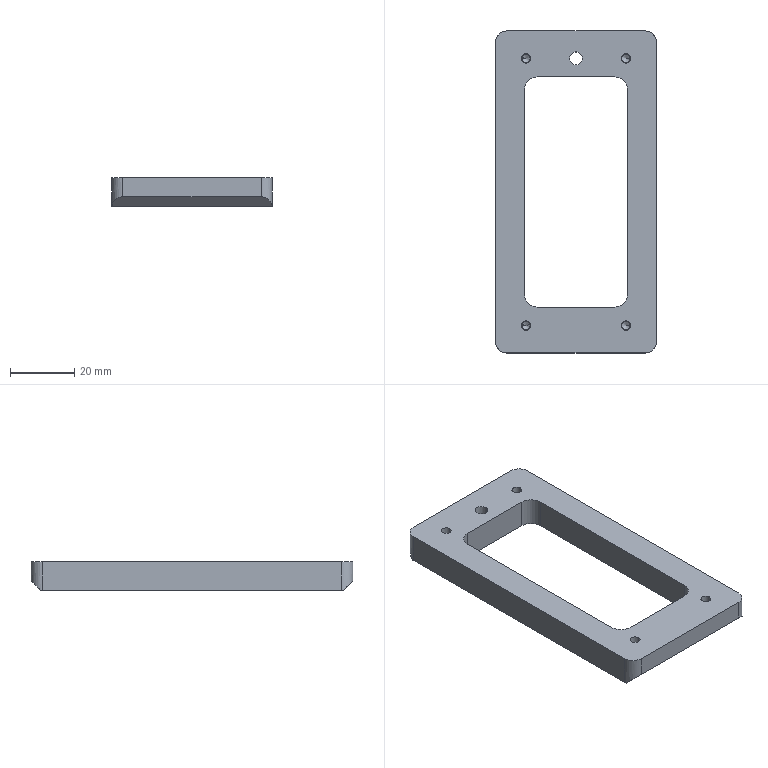Part | STEP file | X77-02213 [2] | 1 solid | 50 faces | box 50 x 100 x 9 mm | volume 23719 mm3 | cylinder 26 | plane 16 | cone 8 | commonest cylinder face diameters 2.5 x8 3 x8 7.116 x4 8 x4 4 x2
STEP:
#1=CARTESIAN_POINT('',(2.,41.5,0.));
#2=VERTEX_POINT('',#1);
#3=CARTESIAN_POINT('',(-2.,41.5,0.));
#4=VERTEX_POINT('',#3);
#5=CARTESIAN_POINT('',(-0.000000005,41.5,0.));
#6=DIRECTION('',(0.,0.,1.));
#7=DIRECTION('',(-1.,0.,0.));
#8=AXIS2_PLACEMENT_3D('',#5,#6,#7);
#9=CIRCLE('',#8,2.);
#10=EDGE_CURVE('',#2,#4,#9,.T.);
#11=ORIENTED_EDGE('',*,*,#10,.F.);
#12=CARTESIAN_POINT('',(2.,41.5,9.));
#13=VERTEX_POINT('',#12);
#14=CARTESIAN_POINT('',(2.,41.5,0.));
#15=DIRECTION('',(0.,0.,1.));
#16=VECTOR('',#15,1000.);
#17=LINE('',#14,#16);
#18=EDGE_CURVE('',#2,#13,#17,.T.);
#19=ORIENTED_EDGE('',*,*,#18,.T.);
#20=CARTESIAN_POINT('',(-2.,41.5,9.));
#21=VERTEX_POINT('',#20);
#22=CARTESIAN_POINT('',(-0.000000005,41.5,9.));
#23=DIRECTION('',(0.,0.,-1.));
#24=DIRECTION('',(-1.,0.,0.));
#25=AXIS2_PLACEMENT_3D('',#22,#23,#24);
#26=CIRCLE('',#25,2.);
#27=EDGE_CURVE('',#21,#13,#26,.T.);
#28=ORIENTED_EDGE('',*,*,#27,.F.);
#29=CARTESIAN_POINT('',(-2.,41.5,0.));
#30=DIRECTION('',(0.,0.,1.));
#31=VECTOR('',#30,1000.);
#32=LINE('',#29,#31);
#33=EDGE_CURVE('',#4,#21,#32,.T.);
#34=ORIENTED_EDGE('',*,*,#33,.F.);
#35=EDGE_LOOP('',(#11,#19,#28,#34));
#36=FACE_OUTER_BOUND('',#35,.T.);
#37=CARTESIAN_POINT('',(-0.000000005,41.5,0.));
#38=DIRECTION('',(0.,0.,1.));
#39=DIRECTION('',(-1.,0.,0.));
#40=AXIS2_PLACEMENT_3D('',#37,#38,#39);
#41=CYLINDRICAL_SURFACE('',#40,2.);
#42=ADVANCED_FACE('',(#36),#41,.F.);
#43=CARTESIAN_POINT('',(-14.001,-41.5,4.));
#44=VERTEX_POINT('',#43);
#45=CARTESIAN_POINT('',(-17.001,-41.5,4.));
#46=VERTEX_POINT('',#45);
#47=CARTESIAN_POINT('',(-15.501,-41.5,4.));
#48=DIRECTION('',(0.,0.,1.));
#49=DIRECTION('',(-1.,0.,0.));
#50=AXIS2_PLACEMENT_3D('',#47,#48,#49);
#51=CIRCLE('',#50,1.5);
#52=EDGE_CURVE('',#44,#46,#51,.T.);
#53=ORIENTED_EDGE('',*,*,#52,.F.);
#54=CARTESIAN_POINT('',(-14.001,-41.5,9.));
#55=VERTEX_POINT('',#54);
#56=CARTESIAN_POINT('',(-14.001,-41.5,10.));
#57=DIRECTION('',(0.,0.,1.));
#58=VECTOR('',#57,1000.);
#59=LINE('',#56,#58);
#60=EDGE_CURVE('',#44,#55,#59,.T.);
#61=ORIENTED_EDGE('',*,*,#60,.T.);
#62=CARTESIAN_POINT('',(-17.001,-41.5,9.));
#63=VERTEX_POINT('',#62);
#64=CARTESIAN_POINT('',(-15.501,-41.5,9.));
#65=DIRECTION('',(0.,0.,-1.));
#66=DIRECTION('',(-1.,0.,0.));
#67=AXIS2_PLACEMENT_3D('',#64,#65,#66);
#68=CIRCLE('',#67,1.5);
#69=EDGE_CURVE('',#63,#55,#68,.T.);
#70=ORIENTED_EDGE('',*,*,#69,.F.);
#71=CARTESIAN_POINT('',(-17.001,-41.5,10.));
#72=DIRECTION('',(0.,0.,1.));
#73=VECTOR('',#72,1000.);
#74=LINE('',#71,#73);
#75=EDGE_CURVE('',#46,#63,#74,.T.);
#76=ORIENTED_EDGE('',*,*,#75,.F.);
#77=EDGE_LOOP('',(#53,#61,#70,#76));
#78=FACE_OUTER_BOUND('',#77,.T.);
#79=CARTESIAN_POINT('',(-15.501,-41.5,10.));
#80=DIRECTION('',(0.,0.,1.));
#81=DIRECTION('',(-1.,0.,0.));
#82=AXIS2_PLACEMENT_3D('',#79,#80,#81);
#83=CYLINDRICAL_SURFACE('',#82,1.5);
#84=ADVANCED_FACE('',(#78),#83,.F.);
#85=CARTESIAN_POINT('',(-14.251,-41.5,2.5));
#86=VERTEX_POINT('',#85);
#87=CARTESIAN_POINT('',(-16.751,-41.5,2.5));
#88=VERTEX_POINT('',#87);
#89=CARTESIAN_POINT('',(-15.501,-41.5,2.5));
#90=DIRECTION('',(0.,0.,1.));
#91=DIRECTION('',(-1.,0.,0.));
#92=AXIS2_PLACEMENT_3D('',#89,#90,#91);
#93=CIRCLE('',#92,1.25);
#94=EDGE_CURVE('',#86,#88,#93,.T.);
#95=ORIENTED_EDGE('',*,*,#94,.F.);
#96=CARTESIAN_POINT('',(-14.251,-41.5,4.));
#97=VERTEX_POINT('',#96);
#98=CARTESIAN_POINT('',(-14.251,-41.5,10.));
#99=DIRECTION('',(0.,0.,1.));
#100=VECTOR('',#99,1000.);
#101=LINE('',#98,#100);
#102=EDGE_CURVE('',#86,#97,#101,.T.);
#103=ORIENTED_EDGE('',*,*,#102,.T.);
#104=CARTESIAN_POINT('',(-16.751,-41.5,4.));
#105=VERTEX_POINT('',#104);
#106=CARTESIAN_POINT('',(-15.501,-41.5,4.));
#107=DIRECTION('',(0.,0.,1.));
#108=DIRECTION('',(-1.,0.,0.));
#109=AXIS2_PLACEMENT_3D('',#106,#107,#108);
#110=CIRCLE('',#109,1.25);
#111=EDGE_CURVE('',#97,#105,#110,.T.);
#112=ORIENTED_EDGE('',*,*,#111,.T.);
#113=CARTESIAN_POINT('',(-16.751,-41.5,10.));
#114=DIRECTION('',(0.,0.,1.));
#115=VECTOR('',#114,1000.);
#116=LINE('',#113,#115);
#117=EDGE_CURVE('',#88,#105,#116,.T.);
#118=ORIENTED_EDGE('',*,*,#117,.F.);
#119=EDGE_LOOP('',(#95,#103,#112,#118));
#120=FACE_OUTER_BOUND('',#119,.T.);
#121=CARTESIAN_POINT('',(-15.501,-41.5,10.));
#122=DIRECTION('',(0.,0.,1.));
#123=DIRECTION('',(-1.,0.,0.));
#124=AXIS2_PLACEMENT_3D('',#121,#122,#123);
#125=CYLINDRICAL_SURFACE('',#124,1.25);
#126=ADVANCED_FACE('',(#120),#125,.F.);
#127=CARTESIAN_POINT('',(-15.501,-41.5,1.749));
#128=VERTEX_POINT('',#127);
#129=CARTESIAN_POINT('',(-16.751,-41.5,2.5));
#130=DIRECTION('',(-0.8572,0.,0.515));
#131=VECTOR('',#130,1000.);
#132=LINE('',#129,#131);
#133=EDGE_CURVE('',#128,#88,#132,.T.);
#134=ORIENTED_EDGE('',*,*,#133,.F.);
#135=CARTESIAN_POINT('',(-14.251,-41.5,2.5));
#136=DIRECTION('',(0.8572,0.,0.515));
#137=VECTOR('',#136,1000.);
#138=LINE('',#135,#137);
#139=EDGE_CURVE('',#128,#86,#138,.T.);
#140=ORIENTED_EDGE('',*,*,#139,.T.);
#141=ORIENTED_EDGE('',*,*,#94,.T.);
#142=EDGE_LOOP('',(#134,#140,#141));
#143=FACE_OUTER_BOUND('',#142,.T.);
#144=CARTESIAN_POINT('',(-15.501,-41.5,2.5));
#145=DIRECTION('',(0.,0.,1.));
#146=DIRECTION('',(-1.,0.,0.));
#147=AXIS2_PLACEMENT_3D('',#144,#145,#146);
#148=CONICAL_SURFACE('',#147,1.25,1.03);
#149=ADVANCED_FACE('',(#143),#148,.F.);
#150=CARTESIAN_POINT('',(-14.005,41.5,4.));
#151=VERTEX_POINT('',#150);
#152=CARTESIAN_POINT('',(-17.005,41.5,4.));
#153=VERTEX_POINT('',#152);
#154=CARTESIAN_POINT('',(-15.505,41.5,4.));
#155=DIRECTION('',(0.,0.,1.));
#156=DIRECTION('',(-1.,0.,0.));
#157=AXIS2_PLACEMENT_3D('',#154,#155,#156);
#158=CIRCLE('',#157,1.5);
#159=EDGE_CURVE('',#151,#153,#158,.T.);
#160=ORIENTED_EDGE('',*,*,#159,.F.);
#161=CARTESIAN_POINT('',(-14.005,41.5,9.));
#162=VERTEX_POINT('',#161);
#163=CARTESIAN_POINT('',(-14.005,41.5,10.));
#164=DIRECTION('',(0.,0.,1.));
#165=VECTOR('',#164,1000.);
#166=LINE('',#163,#165);
#167=EDGE_CURVE('',#151,#162,#166,.T.);
#168=ORIENTED_EDGE('',*,*,#167,.T.);
#169=CARTESIAN_POINT('',(-17.005,41.5,9.));
#170=VERTEX_POINT('',#169);
#171=CARTESIAN_POINT('',(-15.505,41.5,9.));
#172=DIRECTION('',(0.,0.,-1.));
#173=DIRECTION('',(-1.,0.,0.));
#174=AXIS2_PLACEMENT_3D('',#171,#172,#173);
#175=CIRCLE('',#174,1.5);
#176=EDGE_CURVE('',#170,#162,#175,.T.);
#177=ORIENTED_EDGE('',*,*,#176,.F.);
#178=CARTESIAN_POINT('',(-17.005,41.5,10.));
#179=DIRECTION('',(0.,0.,1.));
#180=VECTOR('',#179,1000.);
#181=LINE('',#178,#180);
#182=EDGE_CURVE('',#153,#170,#181,.T.);
#183=ORIENTED_EDGE('',*,*,#182,.F.);
#184=EDGE_LOOP('',(#160,#168,#177,#183));
#185=FACE_OUTER_BOUND('',#184,.T.);
#186=CARTESIAN_POINT('',(-15.505,41.5,10.));
#187=DIRECTION('',(0.,0.,1.));
#188=DIRECTION('',(-1.,0.,0.));
#189=AXIS2_PLACEMENT_3D('',#186,#187,#188);
#190=CYLINDRICAL_SURFACE('',#189,1.5);
#191=ADVANCED_FACE('',(#185),#190,.F.);
#192=CARTESIAN_POINT('',(-14.255,41.5,2.5));
#193=VERTEX_POINT('',#192);
#194=CARTESIAN_POINT('',(-16.755,41.5,2.5));
#195=VERTEX_POINT('',#194);
#196=CARTESIAN_POINT('',(-15.505,41.5,2.5));
#197=DIRECTION('',(0.,0.,1.));
#198=DIRECTION('',(-1.,0.,0.));
#199=AXIS2_PLACEMENT_3D('',#196,#197,#198);
#200=CIRCLE('',#199,1.25);
#201=EDGE_CURVE('',#193,#195,#200,.T.);
#202=ORIENTED_EDGE('',*,*,#201,.F.);
#203=CARTESIAN_POINT('',(-14.255,41.5,4.));
#204=VERTEX_POINT('',#203);
#205=CARTESIAN_POINT('',(-14.255,41.5,10.));
#206=DIRECTION('',(0.,0.,1.));
#207=VECTOR('',#206,1000.);
#208=LINE('',#205,#207);
#209=EDGE_CURVE('',#193,#204,#208,.T.);
#210=ORIENTED_EDGE('',*,*,#209,.T.);
#211=CARTESIAN_POINT('',(-16.755,41.5,4.));
#212=VERTEX_POINT('',#211);
#213=CARTESIAN_POINT('',(-15.505,41.5,4.));
#214=DIRECTION('',(0.,0.,1.));
#215=DIRECTION('',(-1.,0.,0.));
#216=AXIS2_PLACEMENT_3D('',#213,#214,#215);
#217=CIRCLE('',#216,1.25);
#218=EDGE_CURVE('',#204,#212,#217,.T.);
#219=ORIENTED_EDGE('',*,*,#218,.T.);
#220=CARTESIAN_POINT('',(-16.755,41.5,10.));
#221=DIRECTION('',(0.,0.,1.));
#222=VECTOR('',#221,1000.);
#223=LINE('',#220,#222);
#224=EDGE_CURVE('',#195,#212,#223,.T.);
#225=ORIENTED_EDGE('',*,*,#224,.F.);
#226=EDGE_LOOP('',(#202,#210,#219,#225));
#227=FACE_OUTER_BOUND('',#226,.T.);
#228=CARTESIAN_POINT('',(-15.505,41.5,10.));
#229=DIRECTION('',(0.,0.,1.));
#230=DIRECTION('',(-1.,0.,0.));
#231=AXIS2_PLACEMENT_3D('',#228,#229,#230);
#232=CYLINDRICAL_SURFACE('',#231,1.25);
#233=ADVANCED_FACE('',(#227),#232,.F.);
#234=CARTESIAN_POINT('',(-15.505,41.5,1.749));
#235=VERTEX_POINT('',#234);
#236=CARTESIAN_POINT('',(-16.755,41.5,2.5));
#237=DIRECTION('',(-0.8572,0.,0.515));
#238=VECTOR('',#237,1000.);
#239=LINE('',#236,#238);
#240=EDGE_CURVE('',#235,#195,#239,.T.);
#241=ORIENTED_EDGE('',*,*,#240,.F.);
#242=CARTESIAN_POINT('',(-14.255,41.5,2.5));
#243=DIRECTION('',(0.8572,0.,0.515));
#244=VECTOR('',#243,1000.);
#245=LINE('',#242,#244);
#246=EDGE_CURVE('',#235,#193,#245,.T.);
#247=ORIENTED_EDGE('',*,*,#246,.T.);
#248=ORIENTED_EDGE('',*,*,#201,.T.);
#249=EDGE_LOOP('',(#241,#247,#248));
#250=FACE_OUTER_BOUND('',#249,.T.);
#251=CARTESIAN_POINT('',(-15.505,41.5,2.5));
#252=DIRECTION('',(0.,0.,1.));
#253=DIRECTION('',(-1.,0.,0.));
#254=AXIS2_PLACEMENT_3D('',#251,#252,#253);
#255=CONICAL_SURFACE('',#254,1.25,1.03);
#256=ADVANCED_FACE('',(#250),#255,.F.);
#257=CARTESIAN_POINT('',(16.999,41.5,4.));
#258=VERTEX_POINT('',#257);
#259=CARTESIAN_POINT('',(13.999,41.5,4.));
#260=VERTEX_POINT('',#259);
#261=CARTESIAN_POINT('',(15.499,41.5,4.));
#262=DIRECTION('',(0.,0.,1.));
#263=DIRECTION('',(-1.,0.,0.));
#264=AXIS2_PLACEMENT_3D('',#261,#262,#263);
#265=CIRCLE('',#264,1.5);
#266=EDGE_CURVE('',#258,#260,#265,.T.);
#267=ORIENTED_EDGE('',*,*,#266,.F.);
#268=CARTESIAN_POINT('',(16.999,41.5,9.));
#269=VERTEX_POINT('',#268);
#270=CARTESIAN_POINT('',(16.999,41.5,10.));
#271=DIRECTION('',(0.,0.,1.));
#272=VECTOR('',#271,1000.);
#273=LINE('',#270,#272);
#274=EDGE_CURVE('',#258,#269,#273,.T.);
#275=ORIENTED_EDGE('',*,*,#274,.T.);
#276=CARTESIAN_POINT('',(13.999,41.5,9.));
#277=VERTEX_POINT('',#276);
#278=CARTESIAN_POINT('',(15.499,41.5,9.));
#279=DIRECTION('',(0.,0.,-1.));
#280=DIRECTION('',(-1.,0.,0.));
#281=AXIS2_PLACEMENT_3D('',#278,#279,#280);
#282=CIRCLE('',#281,1.5);
#283=EDGE_CURVE('',#277,#269,#282,.T.);
#284=ORIENTED_EDGE('',*,*,#283,.F.);
#285=CARTESIAN_POINT('',(13.999,41.5,10.));
#286=DIRECTION('',(0.,0.,1.));
#287=VECTOR('',#286,1000.);
#288=LINE('',#285,#287);
#289=EDGE_CURVE('',#260,#277,#288,.T.);
#290=ORIENTED_EDGE('',*,*,#289,.F.);
#291=EDGE_LOOP('',(#267,#275,#284,#290));
#292=FACE_OUTER_BOUND('',#291,.T.);
#293=CARTESIAN_POINT('',(15.499,41.5,10.));
#294=DIRECTION('',(0.,0.,1.));
#295=DIRECTION('',(-1.,0.,0.));
#296=AXIS2_PLACEMENT_3D('',#293,#294,#295);
#297=CYLINDRICAL_SURFACE('',#296,1.5);
#298=ADVANCED_FACE('',(#292),#297,.F.);
#299=CARTESIAN_POINT('',(16.749,41.5,2.5));
#300=VERTEX_POINT('',#299);
#301=CARTESIAN_POINT('',(14.249,41.5,2.5));
#302=VERTEX_POINT('',#301);
#303=CARTESIAN_POINT('',(15.499,41.5,2.5));
#304=DIRECTION('',(0.,0.,1.));
#305=DIRECTION('',(-1.,0.,0.));
#306=AXIS2_PLACEMENT_3D('',#303,#304,#305);
#307=CIRCLE('',#306,1.25);
#308=EDGE_CURVE('',#300,#302,#307,.T.);
#309=ORIENTED_EDGE('',*,*,#308,.F.);
#310=CARTESIAN_POINT('',(16.749,41.5,4.));
#311=VERTEX_POINT('',#310);
#312=CARTESIAN_POINT('',(16.749,41.5,10.));
#313=DIRECTION('',(0.,0.,1.));
#314=VECTOR('',#313,1000.);
#315=LINE('',#312,#314);
#316=EDGE_CURVE('',#300,#311,#315,.T.);
#317=ORIENTED_EDGE('',*,*,#316,.T.);
#318=CARTESIAN_POINT('',(14.249,41.5,4.));
#319=VERTEX_POINT('',#318);
#320=CARTESIAN_POINT('',(15.499,41.5,4.));
#321=DIRECTION('',(0.,0.,1.));
#322=DIRECTION('',(-1.,0.,0.));
#323=AXIS2_PLACEMENT_3D('',#320,#321,#322);
#324=CIRCLE('',#323,1.25);
#325=EDGE_CURVE('',#311,#319,#324,.T.);
#326=ORIENTED_EDGE('',*,*,#325,.T.);
#327=CARTESIAN_POINT('',(14.249,41.5,10.));
#328=DIRECTION('',(0.,0.,1.));
#329=VECTOR('',#328,1000.);
#330=LINE('',#327,#329);
#331=EDGE_CURVE('',#302,#319,#330,.T.);
#332=ORIENTED_EDGE('',*,*,#331,.F.);
#333=EDGE_LOOP('',(#309,#317,#326,#332));
#334=FACE_OUTER_BOUND('',#333,.T.);
#335=CARTESIAN_POINT('',(15.499,41.5,10.));
#336=DIRECTION('',(0.,0.,1.));
#337=DIRECTION('',(-1.,0.,0.));
#338=AXIS2_PLACEMENT_3D('',#335,#336,#337);
#339=CYLINDRICAL_SURFACE('',#338,1.25);
#340=ADVANCED_FACE('',(#334),#339,.F.);
#341=CARTESIAN_POINT('',(15.499,41.5,1.749));
#342=VERTEX_POINT('',#341);
#343=CARTESIAN_POINT('',(14.249,41.5,2.5));
#344=DIRECTION('',(-0.8572,0.,0.515));
#345=VECTOR('',#344,1000.);
#346=LINE('',#343,#345);
#347=EDGE_CURVE('',#342,#302,#346,.T.);
#348=ORIENTED_EDGE('',*,*,#347,.F.);
#349=CARTESIAN_POINT('',(16.749,41.5,2.5));
#350=DIRECTION('',(0.8572,0.,0.515));
#351=VECTOR('',#350,1000.);
#352=LINE('',#349,#351);
#353=EDGE_CURVE('',#342,#300,#352,.T.);
#354=ORIENTED_EDGE('',*,*,#353,.T.);
#355=ORIENTED_EDGE('',*,*,#308,.T.);
#356=EDGE_LOOP('',(#348,#354,#355));
#357=FACE_OUTER_BOUND('',#356,.T.);
#358=CARTESIAN_POINT('',(15.499,41.5,2.5));
#359=DIRECTION('',(0.,0.,1.));
#360=DIRECTION('',(-1.,0.,0.));
#361=AXIS2_PLACEMENT_3D('',#358,#359,#360);
#362=CONICAL_SURFACE('',#361,1.25,1.03);
#363=ADVANCED_FACE('',(#357),#362,.F.);
#364=CARTESIAN_POINT('',(16.75,-41.5,2.5));
#365=VERTEX_POINT('',#364);
#366=CARTESIAN_POINT('',(14.25,-41.5,2.5));
#367=VERTEX_POINT('',#366);
#368=CARTESIAN_POINT('',(15.5,-41.5,2.5));
#369=DIRECTION('',(0.,0.,1.));
#370=DIRECTION('',(-1.,0.,0.));
#371=AXIS2_PLACEMENT_3D('',#368,#369,#370);
#372=CIRCLE('',#371,1.25);
#373=EDGE_CURVE('',#365,#367,#372,.T.);
#374=ORIENTED_EDGE('',*,*,#373,.F.);
#375=CARTESIAN_POINT('',(16.75,-41.5,4.));
#376=VERTEX_POINT('',#375);
#377=CARTESIAN_POINT('',(16.75,-41.5,10.));
#378=DIRECTION('',(0.,0.,1.));
#379=VECTOR('',#378,1000.);
#380=LINE('',#377,#379);
#381=EDGE_CURVE('',#365,#376,#380,.T.);
#382=ORIENTED_EDGE('',*,*,#381,.T.);
#383=CARTESIAN_POINT('',(14.25,-41.5,4.));
#384=VERTEX_POINT('',#383);
#385=CARTESIAN_POINT('',(15.5,-41.5,4.));
#386=DIRECTION('',(0.,0.,1.));
#387=DIRECTION('',(-1.,0.,0.));
#388=AXIS2_PLACEMENT_3D('',#385,#386,#387);
#389=CIRCLE('',#388,1.25);
#390=EDGE_CURVE('',#376,#384,#389,.T.);
#391=ORIENTED_EDGE('',*,*,#390,.T.);
#392=CARTESIAN_POINT('',(14.25,-41.5,10.));
#393=DIRECTION('',(0.,0.,1.));
#394=VECTOR('',#393,1000.);
#395=LINE('',#392,#394);
#396=EDGE_CURVE('',#367,#384,#395,.T.);
#397=ORIENTED_EDGE('',*,*,#396,.F.);
#398=EDGE_LOOP('',(#374,#382,#391,#397));
#399=FACE_OUTER_BOUND('',#398,.T.);
#400=CARTESIAN_POINT('',(15.5,-41.5,10.));
#401=DIRECTION('',(0.,0.,1.));
#402=DIRECTION('',(-1.,0.,0.));
#403=AXIS2_PLACEMENT_3D('',#400,#401,#402);
#404=CYLINDRICAL_SURFACE('',#403,1.25);
#405=ADVANCED_FACE('',(#399),#404,.F.);
#406=CARTESIAN_POINT('',(15.5,-41.5,1.749));
#407=VERTEX_POINT('',#406);
#408=CARTESIAN_POINT('',(14.25,-41.5,2.5));
#409=DIRECTION('',(-0.8572,0.,0.515));
#410=VECTOR('',#409,1000.);
#411=LINE('',#408,#410);
#412=EDGE_CURVE('',#407,#367,#411,.T.);
#413=ORIENTED_EDGE('',*,*,#412,.F.);
#414=CARTESIAN_POINT('',(16.75,-41.5,2.5));
#415=DIRECTION('',(0.8572,0.,0.515));
#416=VECTOR('',#415,1000.);
#417=LINE('',#414,#416);
#418=EDGE_CURVE('',#407,#365,#417,.T.);
#419=ORIENTED_EDGE('',*,*,#418,.T.);
#420=ORIENTED_EDGE('',*,*,#373,.T.);
#421=EDGE_LOOP('',(#413,#419,#420));
#422=FACE_OUTER_BOUND('',#421,.T.);
#423=CARTESIAN_POINT('',(15.5,-41.5,2.5));
#424=DIRECTION('',(0.,0.,1.));
#425=DIRECTION('',(-1.,0.,0.));
#426=AXIS2_PLACEMENT_3D('',#423,#424,#425);
#427=CONICAL_SURFACE('',#426,1.25,1.03);
#428=ADVANCED_FACE('',(#422),#427,.F.);
#429=CARTESIAN_POINT('',(17.,-41.5,4.));
#430=VERTEX_POINT('',#429);
#431=CARTESIAN_POINT('',(14.,-41.5,4.));
#432=VERTEX_POINT('',#431);
#433=CARTESIAN_POINT('',(15.5,-41.5,4.));
#434=DIRECTION('',(0.,0.,1.));
#435=DIRECTION('',(-1.,0.,0.));
#436=AXIS2_PLACEMENT_3D('',#433,#434,#435);
#437=CIRCLE('',#436,1.5);
#438=EDGE_CURVE('',#430,#432,#437,.T.);
#439=ORIENTED_EDGE('',*,*,#438,.F.);
#440=CARTESIAN_POINT('',(17.,-41.5,9.));
#441=VERTEX_POINT('',#440);
#442=CARTESIAN_POINT('',(17.,-41.5,10.));
#443=DIRECTION('',(0.,0.,1.));
#444=VECTOR('',#443,1000.);
#445=LINE('',#442,#444);
#446=EDGE_CURVE('',#430,#441,#445,.T.);
#447=ORIENTED_EDGE('',*,*,#446,.T.);
#448=CARTESIAN_POINT('',(14.,-41.5,9.));
#449=VERTEX_POINT('',#448);
#450=CARTESIAN_POINT('',(15.5,-41.5,9.));
#451=DIRECTION('',(0.,0.,-1.));
#452=DIRECTION('',(-1.,0.,0.));
#453=AXIS2_PLACEMENT_3D('',#450,#451,#452);
#454=CIRCLE('',#453,1.5);
#455=EDGE_CURVE('',#449,#441,#454,.T.);
#456=ORIENTED_EDGE('',*,*,#455,.F.);
#457=CARTESIAN_POINT('',(14.,-41.5,10.));
#458=DIRECTION('',(0.,0.,1.));
#459=VECTOR('',#458,1000.);
#460=LINE('',#457,#459);
#461=EDGE_CURVE('',#432,#449,#460,.T.);
#462=ORIENTED_EDGE('',*,*,#461,.F.);
#463=EDGE_LOOP('',(#439,#447,#456,#462));
#464=FACE_OUTER_BOUND('',#463,.T.);
#465=CARTESIAN_POINT('',(15.5,-41.5,10.));
#466=DIRECTION('',(0.,0.,1.));
#467=DIRECTION('',(-1.,0.,0.));
#468=AXIS2_PLACEMENT_3D('',#465,#466,#467);
#469=CYLINDRICAL_SURFACE('',#468,1.5);
#470=ADVANCED_FACE('',(#464),#469,.F.);
#471=ORIENTED_EDGE('',*,*,#446,.F.);
#472=CARTESIAN_POINT('',(15.5,-41.5,4.));
#473=DIRECTION('',(0.,0.,1.));
#474=DIRECTION('',(-1.,0.,0.));
#475=AXIS2_PLACEMENT_3D('',#472,#473,#474);
#476=CIRCLE('',#475,1.5);
#477=EDGE_CURVE('',#432,#430,#476,.T.);
#478=ORIENTED_EDGE('',*,*,#477,.F.);
#479=ORIENTED_EDGE('',*,*,#461,.T.);
#480=CARTESIAN_POINT('',(15.5,-41.5,9.));
#481=DIRECTION('',(0.,0.,-1.));
#482=DIRECTION('',(-1.,0.,0.));
#483=AXIS2_PLACEMENT_3D('',#480,#481,#482);
#484=CIRCLE('',#483,1.5);
#485=EDGE_CURVE('',#441,#449,#484,.T.);
#486=ORIENTED_EDGE('',*,*,#485,.F.);
#487=EDGE_LOOP('',(#471,#478,#479,#486));
#488=FACE_OUTER_BOUND('',#487,.T.);
#489=CARTESIAN_POINT('',(15.5,-41.5,10.));
#490=DIRECTION('',(0.,0.,1.));
#491=DIRECTION('',(-1.,0.,0.));
#492=AXIS2_PLACEMENT_3D('',#489,#490,#491);
#493=CYLINDRICAL_SURFACE('',#492,1.5);
#494=ADVANCED_FACE('',(#488),#493,.F.);
#495=ORIENTED_EDGE('',*,*,#418,.F.);
#496=ORIENTED_EDGE('',*,*,#412,.T.);
#497=CARTESIAN_POINT('',(15.5,-41.5,2.5));
#498=DIRECTION('',(0.,0.,1.));
#499=DIRECTION('',(-1.,0.,0.));
#500=AXIS2_PLACEMENT_3D('',#497,#498,#499);
#501=CIRCLE('',#500,1.25);
#502=EDGE_CURVE('',#367,#365,#501,.T.);
#503=ORIENTED_EDGE('',*,*,#502,.T.);
#504=EDGE_LOOP('',(#495,#496,#503));
#505=FACE_OUTER_BOUND('',#504,.T.);
#506=CARTESIAN_POINT('',(15.5,-41.5,2.5));
#507=DIRECTION('',(0.,0.,1.));
#508=DIRECTION('',(-1.,0.,0.));
#509=AXIS2_PLACEMENT_3D('',#506,#507,#508);
#510=CONICAL_SURFACE('',#509,1.25,1.03);
#511=ADVANCED_FACE('',(#505),#510,.F.);
#512=ORIENTED_EDGE('',*,*,#381,.F.);
#513=ORIENTED_EDGE('',*,*,#502,.F.);
#514=ORIENTED_EDGE('',*,*,#396,.T.);
#515=CARTESIAN_POINT('',(15.5,-41.5,4.));
#516=DIRECTION('',(0.,0.,1.));
#517=DIRECTION('',(-1.,0.,0.));
#518=AXIS2_PLACEMENT_3D('',#515,#516,#517);
#519=CIRCLE('',#518,1.25);
#520=EDGE_CURVE('',#384,#376,#519,.T.);
#521=ORIENTED_EDGE('',*,*,#520,.T.);
#522=EDGE_LOOP('',(#512,#513,#514,#521));
#523=FACE_OUTER_BOUND('',#522,.T.);
#524=CARTESIAN_POINT('',(15.5,-41.5,10.));
#525=DIRECTION('',(0.,0.,1.));
#526=DIRECTION('',(-1.,0.,0.));
#527=AXIS2_PLACEMENT_3D('',#524,#525,#526);
#528=CYLINDRICAL_SURFACE('',#527,1.25);
#529=ADVANCED_FACE('',(#523),#528,.F.);
#530=ORIENTED_EDGE('',*,*,#520,.F.);
#531=ORIENTED_EDGE('',*,*,#390,.F.);
#532=EDGE_LOOP('',(#530,#531));
#533=FACE_BOUND('',#532,.T.);
#534=ORIENTED_EDGE('',*,*,#477,.T.);
#535=ORIENTED_EDGE('',*,*,#438,.T.);
#536=EDGE_LOOP('',(#534,#535));
#537=FACE_OUTER_BOUND('',#536,.T.);
#538=CARTESIAN_POINT('',(15.5,-42.75,4.));
#539=DIRECTION('',(0.,0.,-1.));
#540=DIRECTION('',(1.,0.,0.));
#541=AXIS2_PLACEMENT_3D('',#538,#539,#540);
#542=PLANE('',#541);
#543=ADVANCED_FACE('',(#533,#537),#542,.F.);
#544=ORIENTED_EDGE('',*,*,#455,.T.);
#545=ORIENTED_EDGE('',*,*,#485,.T.);
#546=EDGE_LOOP('',(#544,#545));
#547=FACE_BOUND('',#546,.T.);
#548=ORIENTED_EDGE('',*,*,#69,.T.);
#549=CARTESIAN_POINT('',(-15.501,-41.5,9.));
#550=DIRECTION('',(0.,0.,-1.));
#551=DIRECTION('',(-1.,0.,0.));
#552=AXIS2_PLACEMENT_3D('',#549,#550,#551);
#553=CIRCLE('',#552,1.5);
#554=EDGE_CURVE('',#55,#63,#553,.T.);
#555=ORIENTED_EDGE('',*,*,#554,.T.);
#556=EDGE_LOOP('',(#548,#555));
#557=FACE_BOUND('',#556,.T.);
#558=ORIENTED_EDGE('',*,*,#176,.T.);
#559=CARTESIAN_POINT('',(-15.505,41.5,9.));
#560=DIRECTION('',(0.,0.,-1.));
#561=DIRECTION('',(-1.,0.,0.));
#562=AXIS2_PLACEMENT_3D('',#559,#560,#561);
#563=CIRCLE('',#562,1.5);
#564=EDGE_CURVE('',#162,#170,#563,.T.);
#565=ORIENTED_EDGE('',*,*,#564,.T.);
#566=EDGE_LOOP('',(#558,#565));
#567=FACE_BOUND('',#566,.T.);
#568=ORIENTED_EDGE('',*,*,#283,.T.);
#569=CARTESIAN_POINT('',(15.499,41.5,9.));
#570=DIRECTION('',(0.,0.,-1.));
#571=DIRECTION('',(-1.,0.,0.));
#572=AXIS2_PLACEMENT_3D('',#569,#570,#571);
#573=CIRCLE('',#572,1.5);
#574=EDGE_CURVE('',#269,#277,#573,.T.);
#575=ORIENTED_EDGE('',*,*,#574,.T.);
#576=EDGE_LOOP('',(#568,#575));
#577=FACE_BOUND('',#576,.T.);
#578=ORIENTED_EDGE('',*,*,#27,.T.);
#579=CARTESIAN_POINT('',(-0.000000005,41.5,9.));
#580=DIRECTION('',(0.,0.,-1.));
#581=DIRECTION('',(-1.,0.,0.));
#582=AXIS2_PLACEMENT_3D('',#579,#580,#581);
#583=CIRCLE('',#582,2.);
#584=EDGE_CURVE('',#13,#21,#583,.T.);
#585=ORIENTED_EDGE('',*,*,#584,.T.);
#586=EDGE_LOOP('',(#578,#585));
#587=FACE_BOUND('',#586,.T.);
#588=CARTESIAN_POINT('',(-12.,-35.75,9.));
#589=VERTEX_POINT('',#588);
#590=CARTESIAN_POINT('',(12.,-35.75,9.));
#591=VERTEX_POINT('',#590);
#592=CARTESIAN_POINT('',(-12.,-35.75,9.));
#593=DIRECTION('',(1.,0.,0.));
#594=VECTOR('',#593,1000.);
#595=LINE('',#592,#594);
#596=EDGE_CURVE('',#589,#591,#595,.T.);
#597=ORIENTED_EDGE('',*,*,#596,.F.);
#598=CARTESIAN_POINT('',(-16.,-31.75,9.));
#599=VERTEX_POINT('',#598);
#600=CARTESIAN_POINT('',(-12.,-31.75,9.));
#601=DIRECTION('',(0.,0.,1.));
#602=DIRECTION('',(-1.,0.,0.));
#603=AXIS2_PLACEMENT_3D('',#600,#601,#602);
#604=CIRCLE('',#603,4.);
#605=EDGE_CURVE('',#599,#589,#604,.T.);
#606=ORIENTED_EDGE('',*,*,#605,.F.);
#607=CARTESIAN_POINT('',(-16.,31.75,9.));
#608=VERTEX_POINT('',#607);
#609=CARTESIAN_POINT('',(-16.,-31.75,9.));
#610=DIRECTION('',(0.,-1.,0.));
#611=VECTOR('',#610,1000.);
#612=LINE('',#609,#611);
#613=EDGE_CURVE('',#608,#599,#612,.T.);
#614=ORIENTED_EDGE('',*,*,#613,.F.);
#615=CARTESIAN_POINT('',(-12.,35.75,9.));
#616=VERTEX_POINT('',#615);
#617=CARTESIAN_POINT('',(-12.,31.75,9.));
#618=DIRECTION('',(0.,0.,1.));
#619=DIRECTION('',(-1.,0.,0.));
#620=AXIS2_PLACEMENT_3D('',#617,#618,#619);
#621=CIRCLE('',#620,4.);
#622=EDGE_CURVE('',#616,#608,#621,.T.);
#623=ORIENTED_EDGE('',*,*,#622,.F.);
#624=CARTESIAN_POINT('',(12.,35.75,9.));
#625=VERTEX_POINT('',#624);
#626=CARTESIAN_POINT('',(-12.,35.75,9.));
#627=DIRECTION('',(-1.,0.,0.));
#628=VECTOR('',#627,1000.);
#629=LINE('',#626,#628);
#630=EDGE_CURVE('',#625,#616,#629,.T.);
#631=ORIENTED_EDGE('',*,*,#630,.F.);
#632=CARTESIAN_POINT('',(16.,31.75,9.));
#633=VERTEX_POINT('',#632);
#634=CARTESIAN_POINT('',(12.,31.75,9.));
#635=DIRECTION('',(0.,0.,1.));
#636=DIRECTION('',(-1.,0.,0.));
#637=AXIS2_PLACEMENT_3D('',#634,#635,#636);
#638=CIRCLE('',#637,4.);
#639=EDGE_CURVE('',#633,#625,#638,.T.);
#640=ORIENTED_EDGE('',*,*,#639,.F.);
#641=CARTESIAN_POINT('',(16.,-31.75,9.));
#642=VERTEX_POINT('',#641);
#643=CARTESIAN_POINT('',(16.,-31.75,9.));
#644=DIRECTION('',(0.,1.,0.));
#645=VECTOR('',#644,1000.);
#646=LINE('',#643,#645);
#647=EDGE_CURVE('',#642,#633,#646,.T.);
#648=ORIENTED_EDGE('',*,*,#647,.F.);
#649=CARTESIAN_POINT('',(12.,-31.75,9.));
#650=DIRECTION('',(0.,0.,1.));
#651=DIRECTION('',(-1.,0.,0.));
#652=AXIS2_PLACEMENT_3D('',#649,#650,#651);
#653=CIRCLE('',#652,4.);
#654=EDGE_CURVE('',#591,#642,#653,.T.);
#655=ORIENTED_EDGE('',*,*,#654,.F.);
#656=EDGE_LOOP('',(#597,#606,#614,#623,#631,#640,#648,#655));
#657=FACE_BOUND('',#656,.T.);
#658=CARTESIAN_POINT('',(25.,46.442,9.));
#659=VERTEX_POINT('',#658);
#660=CARTESIAN_POINT('',(21.442,50.,9.));
#661=VERTEX_POINT('',#660);
#662=CARTESIAN_POINT('',(21.442,46.442,9.));
#663=DIRECTION('',(0.,0.,1.));
#664=DIRECTION('',(-1.,0.,0.));
#665=AXIS2_PLACEMENT_3D('',#662,#663,#664);
#666=CIRCLE('',#665,3.558);
#667=EDGE_CURVE('',#659,#661,#666,.T.);
#668=ORIENTED_EDGE('',*,*,#667,.T.);
#669=CARTESIAN_POINT('',(-21.442,50.,9.));
#670=VERTEX_POINT('',#669);
#671=CARTESIAN_POINT('',(-21.442,50.,9.));
#672=DIRECTION('',(-1.,0.,0.));
#673=VECTOR('',#672,1000.);
#674=LINE('',#671,#673);
#675=EDGE_CURVE('',#661,#670,#674,.T.);
#676=ORIENTED_EDGE('',*,*,#675,.T.);
#677=CARTESIAN_POINT('',(-25.,46.442,9.));
#678=VERTEX_POINT('',#677);
#679=CARTESIAN_POINT('',(-21.442,46.442,9.));
#680=DIRECTION('',(0.,0.,1.));
#681=DIRECTION('',(-1.,0.,0.));
#682=AXIS2_PLACEMENT_3D('',#679,#680,#681);
#683=CIRCLE('',#682,3.558);
#684=EDGE_CURVE('',#670,#678,#683,.T.);
#685=ORIENTED_EDGE('',*,*,#684,.T.);
#686=CARTESIAN_POINT('',(-25.,-46.442,9.));
#687=VERTEX_POINT('',#686);
#688=CARTESIAN_POINT('',(-25.,46.442,9.));
#689=DIRECTION('',(0.,-1.,0.));
#690=VECTOR('',#689,1000.);
#691=LINE('',#688,#690);
#692=EDGE_CURVE('',#678,#687,#691,.T.);
#693=ORIENTED_EDGE('',*,*,#692,.T.);
#694=CARTESIAN_POINT('',(-21.442,-50.,9.));
#695=VERTEX_POINT('',#694);
#696=CARTESIAN_POINT('',(-21.442,-46.442,9.));
#697=DIRECTION('',(0.,0.,1.));
#698=DIRECTION('',(-1.,0.,0.));
#699=AXIS2_PLACEMENT_3D('',#696,#697,#698);
#700=CIRCLE('',#699,3.558);
#701=EDGE_CURVE('',#687,#695,#700,.T.);
#702=ORIENTED_EDGE('',*,*,#701,.T.);
#703=CARTESIAN_POINT('',(21.442,-50.,9.));
#704=VERTEX_POINT('',#703);
#705=CARTESIAN_POINT('',(-21.442,-50.,9.));
#706=DIRECTION('',(1.,0.,0.));
#707=VECTOR('',#706,1000.);
#708=LINE('',#705,#707);
#709=EDGE_CURVE('',#695,#704,#708,.T.);
#710=ORIENTED_EDGE('',*,*,#709,.T.);
#711=CARTESIAN_POINT('',(25.,-46.442,9.));
#712=VERTEX_POINT('',#711);
#713=CARTESIAN_POINT('',(21.442,-46.442,9.));
#714=DIRECTION('',(0.,0.,1.));
#715=DIRECTION('',(-1.,0.,0.));
#716=AXIS2_PLACEMENT_3D('',#713,#714,#715);
#717=CIRCLE('',#716,3.558);
#718=EDGE_CURVE('',#704,#712,#717,.T.);
#719=ORIENTED_EDGE('',*,*,#718,.T.);
#720=CARTESIAN_POINT('',(25.,46.442,9.));
#721=DIRECTION('',(0.,1.,0.));
#722=VECTOR('',#721,1000.);
#723=LINE('',#720,#722);
#724=EDGE_CURVE('',#712,#659,#723,.T.);
#725=ORIENTED_EDGE('',*,*,#724,.T.);
#726=EDGE_LOOP('',(#668,#676,#685,#693,#702,#710,#719,#725));
#727=FACE_OUTER_BOUND('',#726,.T.);
#728=CARTESIAN_POINT('',(45.,53.063,9.));
#729=DIRECTION('',(0.,0.,1.));
#730=DIRECTION('',(-1.,0.,0.));
#731=AXIS2_PLACEMENT_3D('',#728,#729,#730);
#732=PLANE('',#731);
#733=ADVANCED_FACE('',(#547,#557,#567,#577,#587,#657,#727),#732,.T.);
#734=ORIENTED_EDGE('',*,*,#353,.F.);
#735=ORIENTED_EDGE('',*,*,#347,.T.);
#736=CARTESIAN_POINT('',(15.499,41.5,2.5));
#737=DIRECTION('',(0.,0.,1.));
#738=DIRECTION('',(-1.,0.,0.));
#739=AXIS2_PLACEMENT_3D('',#736,#737,#738);
#740=CIRCLE('',#739,1.25);
#741=EDGE_CURVE('',#302,#300,#740,.T.);
#742=ORIENTED_EDGE('',*,*,#741,.T.);
#743=EDGE_LOOP('',(#734,#735,#742));
#744=FACE_OUTER_BOUND('',#743,.T.);
#745=CARTESIAN_POINT('',(15.499,41.5,2.5));
#746=DIRECTION('',(0.,0.,1.));
#747=DIRECTION('',(-1.,0.,0.));
#748=AXIS2_PLACEMENT_3D('',#745,#746,#747);
#749=CONICAL_SURFACE('',#748,1.25,1.03);
#750=ADVANCED_FACE('',(#744),#749,.F.);
#751=ORIENTED_EDGE('',*,*,#316,.F.);
#752=ORIENTED_EDGE('',*,*,#741,.F.);
#753=ORIENTED_EDGE('',*,*,#331,.T.);
#754=CARTESIAN_POINT('',(15.499,41.5,4.));
#755=DIRECTION('',(0.,0.,1.));
#756=DIRECTION('',(-1.,0.,0.));
#757=AXIS2_PLACEMENT_3D('',#754,#755,#756);
#758=CIRCLE('',#757,1.25);
#759=EDGE_CURVE('',#319,#311,#758,.T.);
#760=ORIENTED_EDGE('',*,*,#759,.T.);
#761=EDGE_LOOP('',(#751,#752,#753,#760));
#762=FACE_OUTER_BOUND('',#761,.T.);
#763=CARTESIAN_POINT('',(15.499,41.5,10.));
#764=DIRECTION('',(0.,0.,1.));
#765=DIRECTION('',(-1.,0.,0.));
#766=AXIS2_PLACEMENT_3D('',#763,#764,#765);
#767=CYLINDRICAL_SURFACE('',#766,1.25);
#768=ADVANCED_FACE('',(#762),#767,.F.);
#769=ORIENTED_EDGE('',*,*,#759,.F.);
#770=ORIENTED_EDGE('',*,*,#325,.F.);
#771=EDGE_LOOP('',(#769,#770));
#772=FACE_BOUND('',#771,.T.);
#773=CARTESIAN_POINT('',(15.499,41.5,4.));
#774=DIRECTION('',(0.,0.,1.));
#775=DIRECTION('',(-1.,0.,0.));
#776=AXIS2_PLACEMENT_3D('',#773,#774,#775);
#777=CIRCLE('',#776,1.5);
#778=EDGE_CURVE('',#260,#258,#777,.T.);
#779=ORIENTED_EDGE('',*,*,#778,.T.);
#780=ORIENTED_EDGE('',*,*,#266,.T.);
#781=EDGE_LOOP('',(#779,#780));
#782=FACE_OUTER_BOUND('',#781,.T.);
#783=CARTESIAN_POINT('',(15.499,40.25,4.));
#784=DIRECTION('',(0.,0.,-1.));
#785=DIRECTION('',(1.,0.,0.));
#786=AXIS2_PLACEMENT_3D('',#783,#784,#785);
#787=PLANE('',#786);
#788=ADVANCED_FACE('',(#772,#782),#787,.F.);
#789=ORIENTED_EDGE('',*,*,#274,.F.);
#790=ORIENTED_EDGE('',*,*,#778,.F.);
#791=ORIENTED_EDGE('',*,*,#289,.T.);
#792=ORIENTED_EDGE('',*,*,#574,.F.);
#793=EDGE_LOOP('',(#789,#790,#791,#792));
#794=FACE_OUTER_BOUND('',#793,.T.);
#795=CARTESIAN_POINT('',(15.499,41.5,10.));
#796=DIRECTION('',(0.,0.,1.));
#797=DIRECTION('',(-1.,0.,0.));
#798=AXIS2_PLACEMENT_3D('',#795,#796,#797);
#799=CYLINDRICAL_SURFACE('',#798,1.5);
#800=ADVANCED_FACE('',(#794),#799,.F.);
#801=ORIENTED_EDGE('',*,*,#246,.F.);
#802=ORIENTED_EDGE('',*,*,#240,.T.);
#803=CARTESIAN_POINT('',(-15.505,41.5,2.5));
#804=DIRECTION('',(0.,0.,1.));
#805=DIRECTION('',(-1.,0.,0.));
#806=AXIS2_PLACEMENT_3D('',#803,#804,#805);
#807=CIRCLE('',#806,1.25);
#808=EDGE_CURVE('',#195,#193,#807,.T.);
#809=ORIENTED_EDGE('',*,*,#808,.T.);
#810=EDGE_LOOP('',(#801,#802,#809));
#811=FACE_OUTER_BOUND('',#810,.T.);
#812=CARTESIAN_POINT('',(-15.505,41.5,2.5));
#813=DIRECTION('',(0.,0.,1.));
#814=DIRECTION('',(-1.,0.,0.));
#815=AXIS2_PLACEMENT_3D('',#812,#813,#814);
#816=CONICAL_SURFACE('',#815,1.25,1.03);
#817=ADVANCED_FACE('',(#811),#816,.F.);
#818=ORIENTED_EDGE('',*,*,#209,.F.);
#819=ORIENTED_EDGE('',*,*,#808,.F.);
#820=ORIENTED_EDGE('',*,*,#224,.T.);
#821=CARTESIAN_POINT('',(-15.505,41.5,4.));
#822=DIRECTION('',(0.,0.,1.));
#823=DIRECTION('',(-1.,0.,0.));
#824=AXIS2_PLACEMENT_3D('',#821,#822,#823);
#825=CIRCLE('',#824,1.25);
#826=EDGE_CURVE('',#212,#204,#825,.T.);
#827=ORIENTED_EDGE('',*,*,#826,.T.);
#828=EDGE_LOOP('',(#818,#819,#820,#827));
#829=FACE_OUTER_BOUND('',#828,.T.);
#830=CARTESIAN_POINT('',(-15.505,41.5,10.));
#831=DIRECTION('',(0.,0.,1.));
#832=DIRECTION('',(-1.,0.,0.));
#833=AXIS2_PLACEMENT_3D('',#830,#831,#832);
#834=CYLINDRICAL_SURFACE('',#833,1.25);
#835=ADVANCED_FACE('',(#829),#834,.F.);
#836=ORIENTED_EDGE('',*,*,#826,.F.);
#837=ORIENTED_EDGE('',*,*,#218,.F.);
#838=EDGE_LOOP('',(#836,#837));
#839=FACE_BOUND('',#838,.T.);
#840=CARTESIAN_POINT('',(-15.505,41.5,4.));
#841=DIRECTION('',(0.,0.,1.));
#842=DIRECTION('',(-1.,0.,0.));
#843=AXIS2_PLACEMENT_3D('',#840,#841,#842);
#844=CIRCLE('',#843,1.5);
#845=EDGE_CURVE('',#153,#151,#844,.T.);
#846=ORIENTED_EDGE('',*,*,#845,.T.);
#847=ORIENTED_EDGE('',*,*,#159,.T.);
#848=EDGE_LOOP('',(#846,#847));
#849=FACE_OUTER_BOUND('',#848,.T.);
#850=CARTESIAN_POINT('',(-15.505,40.25,4.));
#851=DIRECTION('',(0.,0.,-1.));
#852=DIRECTION('',(1.,0.,0.));
#853=AXIS2_PLACEMENT_3D('',#850,#851,#852);
#854=PLANE('',#853);
#855=ADVANCED_FACE('',(#839,#849),#854,.F.);
#856=ORIENTED_EDGE('',*,*,#167,.F.);
#857=ORIENTED_EDGE('',*,*,#845,.F.);
#858=ORIENTED_EDGE('',*,*,#182,.T.);
#859=ORIENTED_EDGE('',*,*,#564,.F.);
#860=EDGE_LOOP('',(#856,#857,#858,#859));
#861=FACE_OUTER_BOUND('',#860,.T.);
#862=CARTESIAN_POINT('',(-15.505,41.5,10.));
#863=DIRECTION('',(0.,0.,1.));
#864=DIRECTION('',(-1.,0.,0.));
#865=AXIS2_PLACEMENT_3D('',#862,#863,#864);
#866=CYLINDRICAL_SURFACE('',#865,1.5);
#867=ADVANCED_FACE('',(#861),#866,.F.);
#868=ORIENTED_EDGE('',*,*,#139,.F.);
#869=ORIENTED_EDGE('',*,*,#133,.T.);
#870=CARTESIAN_POINT('',(-15.501,-41.5,2.5));
#871=DIRECTION('',(0.,0.,1.));
#872=DIRECTION('',(-1.,0.,0.));
#873=AXIS2_PLACEMENT_3D('',#870,#871,#872);
#874=CIRCLE('',#873,1.25);
#875=EDGE_CURVE('',#88,#86,#874,.T.);
#876=ORIENTED_EDGE('',*,*,#875,.T.);
#877=EDGE_LOOP('',(#868,#869,#876));
#878=FACE_OUTER_BOUND('',#877,.T.);
#879=CARTESIAN_POINT('',(-15.501,-41.5,2.5));
#880=DIRECTION('',(0.,0.,1.));
#881=DIRECTION('',(-1.,0.,0.));
#882=AXIS2_PLACEMENT_3D('',#879,#880,#881);
#883=CONICAL_SURFACE('',#882,1.25,1.03);
#884=ADVANCED_FACE('',(#878),#883,.F.);
#885=ORIENTED_EDGE('',*,*,#102,.F.);
#886=ORIENTED_EDGE('',*,*,#875,.F.);
#887=ORIENTED_EDGE('',*,*,#117,.T.);
#888=CARTESIAN_POINT('',(-15.501,-41.5,4.));
#889=DIRECTION('',(0.,0.,1.));
#890=DIRECTION('',(-1.,0.,0.));
#891=AXIS2_PLACEMENT_3D('',#888,#889,#890);
#892=CIRCLE('',#891,1.25);
#893=EDGE_CURVE('',#105,#97,#892,.T.);
#894=ORIENTED_EDGE('',*,*,#893,.T.);
#895=EDGE_LOOP('',(#885,#886,#887,#894));
#896=FACE_OUTER_BOUND('',#895,.T.);
#897=CARTESIAN_POINT('',(-15.501,-41.5,10.));
#898=DIRECTION('',(0.,0.,1.));
#899=DIRECTION('',(-1.,0.,0.));
#900=AXIS2_PLACEMENT_3D('',#897,#898,#899);
#901=CYLINDRICAL_SURFACE('',#900,1.25);
#902=ADVANCED_FACE('',(#896),#901,.F.);
#903=ORIENTED_EDGE('',*,*,#893,.F.);
#904=ORIENTED_EDGE('',*,*,#111,.F.);
#905=EDGE_LOOP('',(#903,#904));
#906=FACE_BOUND('',#905,.T.);
#907=CARTESIAN_POINT('',(-15.501,-41.5,4.));
#908=DIRECTION('',(0.,0.,1.));
#909=DIRECTION('',(-1.,0.,0.));
#910=AXIS2_PLACEMENT_3D('',#907,#908,#909);
#911=CIRCLE('',#910,1.5);
#912=EDGE_CURVE('',#46,#44,#911,.T.);
#913=ORIENTED_EDGE('',*,*,#912,.T.);
#914=ORIENTED_EDGE('',*,*,#52,.T.);
#915=EDGE_LOOP('',(#913,#914));
#916=FACE_OUTER_BOUND('',#915,.T.);
#917=CARTESIAN_POINT('',(-15.501,-42.75,4.));
#918=DIRECTION('',(0.,0.,-1.));
#919=DIRECTION('',(1.,0.,0.));
#920=AXIS2_PLACEMENT_3D('',#917,#918,#919);
#921=PLANE('',#920);
#922=ADVANCED_FACE('',(#906,#916),#921,.F.);
#923=ORIENTED_EDGE('',*,*,#60,.F.);
#924=ORIENTED_EDGE('',*,*,#912,.F.);
#925=ORIENTED_EDGE('',*,*,#75,.T.);
#926=ORIENTED_EDGE('',*,*,#554,.F.);
#927=EDGE_LOOP('',(#923,#924,#925,#926));
#928=FACE_OUTER_BOUND('',#927,.T.);
#929=CARTESIAN_POINT('',(-15.501,-41.5,10.));
#930=DIRECTION('',(0.,0.,1.));
#931=DIRECTION('',(-1.,0.,0.));
#932=AXIS2_PLACEMENT_3D('',#929,#930,#931);
#933=CYLINDRICAL_SURFACE('',#932,1.5);
#934=ADVANCED_FACE('',(#928),#933,.F.);
#935=CARTESIAN_POINT('',(-24.956,47.,0.));
#936=VERTEX_POINT('',#935);
#937=CARTESIAN_POINT('',(24.956,47.,0.));
#938=VERTEX_POINT('',#937);
#939=CARTESIAN_POINT('',(-25.,47.,0.));
#940=DIRECTION('',(1.,0.,0.));
#941=VECTOR('',#940,1000.);
#942=LINE('',#939,#941);
#943=EDGE_CURVE('',#936,#938,#942,.T.);
#944=ORIENTED_EDGE('',*,*,#943,.F.);
#945=CARTESIAN_POINT('',(-21.442,50.,3.));
#946=VERTEX_POINT('',#945);
#947=CARTESIAN_POINT('',(-21.442,50.,3.));
#948=CARTESIAN_POINT('',(-23.275,50.,3.));
#949=CARTESIAN_POINT('',(-24.669,48.81,1.81));
#950=CARTESIAN_POINT('',(-24.956,47.,0.));
#951=(BOUNDED_CURVE()B_SPLINE_CURVE(3,(#947,#948,#949,#950),.UNSPECIFIED.,.F.,.T.)B_SPLINE_CURVE_WITH_KNOTS((4,4),(3.142,4.555),.UNSPECIFIED.)CURVE()GEOMETRIC_REPRESENTATION_ITEM()RATIONAL_B_SPLINE_CURVE((1.,0.8404,0.8404,1.))REPRESENTATION_ITEM(''));
#952=EDGE_CURVE('',#946,#936,#951,.T.);
#953=ORIENTED_EDGE('',*,*,#952,.F.);
#954=CARTESIAN_POINT('',(21.442,50.,3.));
#955=VERTEX_POINT('',#954);
#956=CARTESIAN_POINT('',(-25.,50.,3.));
#957=DIRECTION('',(1.,0.,0.));
#958=VECTOR('',#957,1000.);
#959=LINE('',#956,#958);
#960=EDGE_CURVE('',#946,#955,#959,.T.);
#961=ORIENTED_EDGE('',*,*,#960,.T.);
#962=CARTESIAN_POINT('',(24.956,47.,0.));
#963=CARTESIAN_POINT('',(24.669,48.81,1.81));
#964=CARTESIAN_POINT('',(23.275,50.,3.));
#965=CARTESIAN_POINT('',(21.442,50.,3.));
#966=(BOUNDED_CURVE()B_SPLINE_CURVE(3,(#962,#963,#964,#965),.UNSPECIFIED.,.F.,.F.)B_SPLINE_CURVE_WITH_KNOTS((4,4),(1.728,3.142),.UNSPECIFIED.)CURVE()GEOMETRIC_REPRESENTATION_ITEM()RATIONAL_B_SPLINE_CURVE((1.,0.8404,0.8404,1.))REPRESENTATION_ITEM(''));
#967=EDGE_CURVE('',#938,#955,#966,.T.);
#968=ORIENTED_EDGE('',*,*,#967,.F.);
#969=EDGE_LOOP('',(#944,#953,#961,#968));
#970=FACE_OUTER_BOUND('',#969,.T.);
#971=CARTESIAN_POINT('',(-25.,50.,3.));
#972=DIRECTION('',(0.,-0.7071,0.7071));
#973=DIRECTION('',(0.,-0.7071,-0.7071));
#974=AXIS2_PLACEMENT_3D('',#971,#972,#973);
#975=PLANE('',#974);
#976=ADVANCED_FACE('',(#970),#975,.F.);
#977=CARTESIAN_POINT('',(-24.956,-47.,0.));
#978=VERTEX_POINT('',#977);
#979=CARTESIAN_POINT('',(24.956,-47.,0.));
#980=VERTEX_POINT('',#979);
#981=CARTESIAN_POINT('',(-25.,-47.,0.));
#982=DIRECTION('',(1.,0.,0.));
#983=VECTOR('',#982,1000.);
#984=LINE('',#981,#983);
#985=EDGE_CURVE('',#978,#980,#984,.T.);
#986=ORIENTED_EDGE('',*,*,#985,.T.);
#987=CARTESIAN_POINT('',(21.442,-50.,3.));
#988=VERTEX_POINT('',#987);
#989=CARTESIAN_POINT('',(21.442,-50.,3.));
#990=CARTESIAN_POINT('',(23.275,-50.,3.));
#991=CARTESIAN_POINT('',(24.669,-48.81,1.81));
#992=CARTESIAN_POINT('',(24.956,-47.,0.));
#993=(BOUNDED_CURVE()B_SPLINE_CURVE(3,(#989,#990,#991,#992),.UNSPECIFIED.,.F.,.F.)B_SPLINE_CURVE_WITH_KNOTS((4,4),(3.142,4.555),.UNSPECIFIED.)CURVE()GEOMETRIC_REPRESENTATION_ITEM()RATIONAL_B_SPLINE_CURVE((1.,0.8404,0.8404,1.))REPRESENTATION_ITEM(''));
#994=EDGE_CURVE('',#988,#980,#993,.T.);
#995=ORIENTED_EDGE('',*,*,#994,.F.);
#996=CARTESIAN_POINT('',(-21.442,-50.,3.));
#997=VERTEX_POINT('',#996);
#998=CARTESIAN_POINT('',(-25.,-50.,3.));
#999=DIRECTION('',(1.,0.,0.));
#1000=VECTOR('',#999,1000.);
#1001=LINE('',#998,#1000);
#1002=EDGE_CURVE('',#997,#988,#1001,.T.);
#1003=ORIENTED_EDGE('',*,*,#1002,.F.);
#1004=CARTESIAN_POINT('',(-24.956,-47.,0.));
#1005=CARTESIAN_POINT('',(-24.669,-48.81,1.81));
#1006=CARTESIAN_POINT('',(-23.275,-50.,3.));
#1007=CARTESIAN_POINT('',(-21.442,-50.,3.));
#1008=(BOUNDED_CURVE()B_SPLINE_CURVE(3,(#1004,#1005,#1006,#1007),.UNSPECIFIED.,.F.,.T.)B_SPLINE_CURVE_WITH_KNOTS((4,4),(1.728,3.142),.UNSPECIFIED.)CURVE()GEOMETRIC_REPRESENTATION_ITEM()RATIONAL_B_SPLINE_CURVE((1.,0.8404,0.8404,1.))REPRESENTATION_ITEM(''));
#1009=EDGE_CURVE('',#978,#997,#1008,.T.);
#1010=ORIENTED_EDGE('',*,*,#1009,.F.);
#1011=EDGE_LOOP('',(#986,#995,#1003,#1010));
#1012=FACE_OUTER_BOUND('',#1011,.T.);
#1013=CARTESIAN_POINT('',(-25.,-50.,3.));
#1014=DIRECTION('',(0.,0.7071,0.7071));
#1015=DIRECTION('',(0.,-0.7071,0.7071));
#1016=AXIS2_PLACEMENT_3D('',#1013,#1014,#1015);
#1017=PLANE('',#1016);
#1018=ADVANCED_FACE('',(#1012),#1017,.F.);
#1019=CARTESIAN_POINT('',(-12.,-35.75,0.));
#1020=VERTEX_POINT('',#1019);
#1021=CARTESIAN_POINT('',(-12.,-35.75,10.));
#1022=DIRECTION('',(0.,0.,-1.));
#1023=VECTOR('',#1022,1000.);
#1024=LINE('',#1021,#1023);
#1025=EDGE_CURVE('',#589,#1020,#1024,.T.);
#1026=ORIENTED_EDGE('',*,*,#1025,.F.);
#1027=ORIENTED_EDGE('',*,*,#596,.T.);
#1028=CARTESIAN_POINT('',(12.,-35.75,0.));
#1029=VERTEX_POINT('',#1028);
#1030=CARTESIAN_POINT('',(12.,-35.75,10.));
#1031=DIRECTION('',(0.,0.,-1.));
#1032=VECTOR('',#1031,1000.);
#1033=LINE('',#1030,#1032);
#1034=EDGE_CURVE('',#591,#1029,#1033,.T.);
#1035=ORIENTED_EDGE('',*,*,#1034,.T.);
#1036=CARTESIAN_POINT('',(-12.,-35.75,0.));
#1037=DIRECTION('',(1.,0.,0.));
#1038=VECTOR('',#1037,1000.);
#1039=LINE('',#1036,#1038);
#1040=EDGE_CURVE('',#1020,#1029,#1039,.T.);
#1041=ORIENTED_EDGE('',*,*,#1040,.F.);
#1042=EDGE_LOOP('',(#1026,#1027,#1035,#1041));
#1043=FACE_OUTER_BOUND('',#1042,.T.);
#1044=CARTESIAN_POINT('',(-12.,-35.75,10.));
#1045=DIRECTION('',(0.,1.,0.));
#1046=DIRECTION('',(-1.,0.,0.));
#1047=AXIS2_PLACEMENT_3D('',#1044,#1045,#1046);
#1048=PLANE('',#1047);
#1049=ADVANCED_FACE('',(#1043),#1048,.T.);
#1050=CARTESIAN_POINT('',(-16.,-31.75,0.));
#1051=VERTEX_POINT('',#1050);
#1052=CARTESIAN_POINT('',(-16.,-31.75,10.));
#1053=DIRECTION('',(0.,0.,-1.));
#1054=VECTOR('',#1053,1000.);
#1055=LINE('',#1052,#1054);
#1056=EDGE_CURVE('',#599,#1051,#1055,.T.);
#1057=ORIENTED_EDGE('',*,*,#1056,.F.);
#1058=ORIENTED_EDGE('',*,*,#605,.T.);
#1059=ORIENTED_EDGE('',*,*,#1025,.T.);
#1060=CARTESIAN_POINT('',(-12.,-31.75,0.));
#1061=DIRECTION('',(0.,0.,1.));
#1062=DIRECTION('',(-1.,0.,0.));
#1063=AXIS2_PLACEMENT_3D('',#1060,#1061,#1062);
#1064=CIRCLE('',#1063,4.);
#1065=EDGE_CURVE('',#1051,#1020,#1064,.T.);
#1066=ORIENTED_EDGE('',*,*,#1065,.F.);
#1067=EDGE_LOOP('',(#1057,#1058,#1059,#1066));
#1068=FACE_OUTER_BOUND('',#1067,.T.);
#1069=CARTESIAN_POINT('',(-12.,-31.75,10.));
#1070=DIRECTION('',(0.,0.,-1.));
#1071=DIRECTION('',(-1.,0.,0.));
#1072=AXIS2_PLACEMENT_3D('',#1069,#1070,#1071);
#1073=CYLINDRICAL_SURFACE('',#1072,4.);
#1074=ADVANCED_FACE('',(#1068),#1073,.F.);
#1075=CARTESIAN_POINT('',(-16.,31.75,0.));
#1076=VERTEX_POINT('',#1075);
#1077=CARTESIAN_POINT('',(-16.,31.75,10.));
#1078=DIRECTION('',(0.,0.,-1.));
#1079=VECTOR('',#1078,1000.);
#1080=LINE('',#1077,#1079);
#1081=EDGE_CURVE('',#608,#1076,#1080,.T.);
#1082=ORIENTED_EDGE('',*,*,#1081,.F.);
#1083=ORIENTED_EDGE('',*,*,#613,.T.);
#1084=ORIENTED_EDGE('',*,*,#1056,.T.);
#1085=CARTESIAN_POINT('',(-16.,-31.75,0.));
#1086=DIRECTION('',(0.,-1.,0.));
#1087=VECTOR('',#1086,1000.);
#1088=LINE('',#1085,#1087);
#1089=EDGE_CURVE('',#1076,#1051,#1088,.T.);
#1090=ORIENTED_EDGE('',*,*,#1089,.F.);
#1091=EDGE_LOOP('',(#1082,#1083,#1084,#1090));
#1092=FACE_OUTER_BOUND('',#1091,.T.);
#1093=CARTESIAN_POINT('',(-16.,-31.75,10.));
#1094=DIRECTION('',(1.,0.,0.));
#1095=DIRECTION('',(0.,1.,0.));
#1096=AXIS2_PLACEMENT_3D('',#1093,#1094,#1095);
#1097=PLANE('',#1096);
#1098=ADVANCED_FACE('',(#1092),#1097,.T.);
#1099=CARTESIAN_POINT('',(-12.,35.75,0.));
#1100=VERTEX_POINT('',#1099);
#1101=CARTESIAN_POINT('',(-12.,35.75,10.));
#1102=DIRECTION('',(0.,0.,-1.));
#1103=VECTOR('',#1102,1000.);
#1104=LINE('',#1101,#1103);
#1105=EDGE_CURVE('',#616,#1100,#1104,.T.);
#1106=ORIENTED_EDGE('',*,*,#1105,.F.);
#1107=ORIENTED_EDGE('',*,*,#622,.T.);
#1108=ORIENTED_EDGE('',*,*,#1081,.T.);
#1109=CARTESIAN_POINT('',(-12.,31.75,0.));
#1110=DIRECTION('',(0.,0.,1.));
#1111=DIRECTION('',(1.,0.,0.));
#1112=AXIS2_PLACEMENT_3D('',#1109,#1110,#1111);
#1113=CIRCLE('',#1112,4.);
#1114=EDGE_CURVE('',#1100,#1076,#1113,.T.);
#1115=ORIENTED_EDGE('',*,*,#1114,.F.);
#1116=EDGE_LOOP('',(#1106,#1107,#1108,#1115));
#1117=FACE_OUTER_BOUND('',#1116,.T.);
#1118=CARTESIAN_POINT('',(-12.,31.75,10.));
#1119=DIRECTION('',(0.,0.,-1.));
#1120=DIRECTION('',(-1.,0.,0.));
#1121=AXIS2_PLACEMENT_3D('',#1118,#1119,#1120);
#1122=CYLINDRICAL_SURFACE('',#1121,4.);
#1123=ADVANCED_FACE('',(#1117),#1122,.F.);
#1124=CARTESIAN_POINT('',(12.,35.75,0.));
#1125=VERTEX_POINT('',#1124);
#1126=CARTESIAN_POINT('',(12.,35.75,10.));
#1127=DIRECTION('',(0.,0.,-1.));
#1128=VECTOR('',#1127,1000.);
#1129=LINE('',#1126,#1128);
#1130=EDGE_CURVE('',#625,#1125,#1129,.T.);
#1131=ORIENTED_EDGE('',*,*,#1130,.F.);
#1132=ORIENTED_EDGE('',*,*,#630,.T.);
#1133=ORIENTED_EDGE('',*,*,#1105,.T.);
#1134=CARTESIAN_POINT('',(-12.,35.75,0.));
#1135=DIRECTION('',(-1.,0.,0.));
#1136=VECTOR('',#1135,1000.);
#1137=LINE('',#1134,#1136);
#1138=EDGE_CURVE('',#1125,#1100,#1137,.T.);
#1139=ORIENTED_EDGE('',*,*,#1138,.F.);
#1140=EDGE_LOOP('',(#1131,#1132,#1133,#1139));
#1141=FACE_OUTER_BOUND('',#1140,.T.);
#1142=CARTESIAN_POINT('',(-12.,35.75,10.));
#1143=DIRECTION('',(0.,-1.,0.));
#1144=DIRECTION('',(1.,0.,0.));
#1145=AXIS2_PLACEMENT_3D('',#1142,#1143,#1144);
#1146=PLANE('',#1145);
#1147=ADVANCED_FACE('',(#1141),#1146,.T.);
#1148=CARTESIAN_POINT('',(16.,31.75,0.));
#1149=VERTEX_POINT('',#1148);
#1150=CARTESIAN_POINT('',(16.,31.75,10.));
#1151=DIRECTION('',(0.,0.,-1.));
#1152=VECTOR('',#1151,1000.);
#1153=LINE('',#1150,#1152);
#1154=EDGE_CURVE('',#633,#1149,#1153,.T.);
#1155=ORIENTED_EDGE('',*,*,#1154,.F.);
#1156=ORIENTED_EDGE('',*,*,#639,.T.);
#1157=ORIENTED_EDGE('',*,*,#1130,.T.);
#1158=CARTESIAN_POINT('',(12.,31.75,0.));
#1159=DIRECTION('',(0.,0.,1.));
#1160=DIRECTION('',(1.,0.,0.));
#1161=AXIS2_PLACEMENT_3D('',#1158,#1159,#1160);
#1162=CIRCLE('',#1161,4.);
#1163=EDGE_CURVE('',#1149,#1125,#1162,.T.);
#1164=ORIENTED_EDGE('',*,*,#1163,.F.);
#1165=EDGE_LOOP('',(#1155,#1156,#1157,#1164));
#1166=FACE_OUTER_BOUND('',#1165,.T.);
#1167=CARTESIAN_POINT('',(12.,31.75,10.));
#1168=DIRECTION('',(0.,0.,-1.));
#1169=DIRECTION('',(-1.,0.,0.));
#1170=AXIS2_PLACEMENT_3D('',#1167,#1168,#1169);
#1171=CYLINDRICAL_SURFACE('',#1170,4.);
#1172=ADVANCED_FACE('',(#1166),#1171,.F.);
#1173=CARTESIAN_POINT('',(16.,-31.75,0.));
#1174=VERTEX_POINT('',#1173);
#1175=CARTESIAN_POINT('',(16.,-31.75,10.));
#1176=DIRECTION('',(0.,0.,-1.));
#1177=VECTOR('',#1176,1000.);
#1178=LINE('',#1175,#1177);
#1179=EDGE_CURVE('',#642,#1174,#1178,.T.);
#1180=ORIENTED_EDGE('',*,*,#1179,.F.);
#1181=ORIENTED_EDGE('',*,*,#647,.T.);
#1182=ORIENTED_EDGE('',*,*,#1154,.T.);
#1183=CARTESIAN_POINT('',(16.,-31.75,0.));
#1184=DIRECTION('',(0.,1.,0.));
#1185=VECTOR('',#1184,1000.);
#1186=LINE('',#1183,#1185);
#1187=EDGE_CURVE('',#1174,#1149,#1186,.T.);
#1188=ORIENTED_EDGE('',*,*,#1187,.F.);
#1189=EDGE_LOOP('',(#1180,#1181,#1182,#1188));
#1190=FACE_OUTER_BOUND('',#1189,.T.);
#1191=CARTESIAN_POINT('',(16.,-31.75,10.));
#1192=DIRECTION('',(-1.,0.,0.));
#1193=DIRECTION('',(0.,-1.,0.));
#1194=AXIS2_PLACEMENT_3D('',#1191,#1192,#1193);
#1195=PLANE('',#1194);
#1196=ADVANCED_FACE('',(#1190),#1195,.T.);
#1197=ORIENTED_EDGE('',*,*,#1034,.F.);
#1198=ORIENTED_EDGE('',*,*,#654,.T.);
#1199=ORIENTED_EDGE('',*,*,#1179,.T.);
#1200=CARTESIAN_POINT('',(12.,-31.75,0.));
#1201=DIRECTION('',(0.,0.,1.));
#1202=DIRECTION('',(-1.,0.,0.));
#1203=AXIS2_PLACEMENT_3D('',#1200,#1201,#1202);
#1204=CIRCLE('',#1203,4.);
#1205=EDGE_CURVE('',#1029,#1174,#1204,.T.);
#1206=ORIENTED_EDGE('',*,*,#1205,.F.);
#1207=EDGE_LOOP('',(#1197,#1198,#1199,#1206));
#1208=FACE_OUTER_BOUND('',#1207,.T.);
#1209=CARTESIAN_POINT('',(12.,-31.75,10.));
#1210=DIRECTION('',(0.,0.,-1.));
#1211=DIRECTION('',(-1.,0.,0.));
#1212=AXIS2_PLACEMENT_3D('',#1209,#1210,#1211);
#1213=CYLINDRICAL_SURFACE('',#1212,4.);
#1214=ADVANCED_FACE('',(#1208),#1213,.F.);
#1215=ORIENTED_EDGE('',*,*,#724,.F.);
#1216=CARTESIAN_POINT('',(25.,-46.442,0.));
#1217=VERTEX_POINT('',#1216);
#1218=CARTESIAN_POINT('',(25.,-46.442,10.));
#1219=DIRECTION('',(0.,0.,-1.));
#1220=VECTOR('',#1219,1000.);
#1221=LINE('',#1218,#1220);
#1222=EDGE_CURVE('',#712,#1217,#1221,.T.);
#1223=ORIENTED_EDGE('',*,*,#1222,.T.);
#1224=CARTESIAN_POINT('',(25.,46.442,0.));
#1225=VERTEX_POINT('',#1224);
#1226=CARTESIAN_POINT('',(25.,46.442,0.));
#1227=DIRECTION('',(0.,1.,0.));
#1228=VECTOR('',#1227,1000.);
#1229=LINE('',#1226,#1228);
#1230=EDGE_CURVE('',#1217,#1225,#1229,.T.);
#1231=ORIENTED_EDGE('',*,*,#1230,.T.);
#1232=CARTESIAN_POINT('',(25.,46.442,10.));
#1233=DIRECTION('',(0.,0.,-1.));
#1234=VECTOR('',#1233,1000.);
#1235=LINE('',#1232,#1234);
#1236=EDGE_CURVE('',#659,#1225,#1235,.T.);
#1237=ORIENTED_EDGE('',*,*,#1236,.F.);
#1238=EDGE_LOOP('',(#1215,#1223,#1231,#1237));
#1239=FACE_OUTER_BOUND('',#1238,.T.);
#1240=CARTESIAN_POINT('',(25.,46.442,10.));
#1241=DIRECTION('',(-1.,0.,0.));
#1242=DIRECTION('',(0.,0.,1.));
#1243=AXIS2_PLACEMENT_3D('',#1240,#1241,#1242);
#1244=PLANE('',#1243);
#1245=ADVANCED_FACE('',(#1239),#1244,.F.);
#1246=ORIENTED_EDGE('',*,*,#718,.F.);
#1247=CARTESIAN_POINT('',(21.442,-50.,10.));
#1248=DIRECTION('',(0.,0.,-1.));
#1249=VECTOR('',#1248,1000.);
#1250=LINE('',#1247,#1249);
#1251=EDGE_CURVE('',#704,#988,#1250,.T.);
#1252=ORIENTED_EDGE('',*,*,#1251,.T.);
#1253=ORIENTED_EDGE('',*,*,#994,.T.);
#1254=CARTESIAN_POINT('',(21.442,-46.442,0.));
#1255=DIRECTION('',(0.,0.,1.));
#1256=DIRECTION('',(1.,0.,0.));
#1257=AXIS2_PLACEMENT_3D('',#1254,#1255,#1256);
#1258=CIRCLE('',#1257,3.558);
#1259=EDGE_CURVE('',#980,#1217,#1258,.T.);
#1260=ORIENTED_EDGE('',*,*,#1259,.T.);
#1261=ORIENTED_EDGE('',*,*,#1222,.F.);
#1262=EDGE_LOOP('',(#1246,#1252,#1253,#1260,#1261));
#1263=FACE_OUTER_BOUND('',#1262,.T.);
#1264=CARTESIAN_POINT('',(21.442,-46.442,10.));
#1265=DIRECTION('',(0.,0.,-1.));
#1266=DIRECTION('',(-1.,0.,0.));
#1267=AXIS2_PLACEMENT_3D('',#1264,#1265,#1266);
#1268=CYLINDRICAL_SURFACE('',#1267,3.558);
#1269=ADVANCED_FACE('',(#1263),#1268,.T.);
#1270=ORIENTED_EDGE('',*,*,#709,.F.);
#1271=CARTESIAN_POINT('',(-21.442,-50.,10.));
#1272=DIRECTION('',(0.,0.,-1.));
#1273=VECTOR('',#1272,1000.);
#1274=LINE('',#1271,#1273);
#1275=EDGE_CURVE('',#695,#997,#1274,.T.);
#1276=ORIENTED_EDGE('',*,*,#1275,.T.);
#1277=ORIENTED_EDGE('',*,*,#1002,.T.);
#1278=ORIENTED_EDGE('',*,*,#1251,.F.);
#1279=EDGE_LOOP('',(#1270,#1276,#1277,#1278));
#1280=FACE_OUTER_BOUND('',#1279,.T.);
#1281=CARTESIAN_POINT('',(-21.442,-50.,10.));
#1282=DIRECTION('',(0.,1.,0.));
#1283=DIRECTION('',(0.,0.,1.));
#1284=AXIS2_PLACEMENT_3D('',#1281,#1282,#1283);
#1285=PLANE('',#1284);
#1286=ADVANCED_FACE('',(#1280),#1285,.F.);
#1287=ORIENTED_EDGE('',*,*,#701,.F.);
#1288=CARTESIAN_POINT('',(-25.,-46.442,0.));
#1289=VERTEX_POINT('',#1288);
#1290=CARTESIAN_POINT('',(-25.,-46.442,10.));
#1291=DIRECTION('',(0.,0.,-1.));
#1292=VECTOR('',#1291,1000.);
#1293=LINE('',#1290,#1292);
#1294=EDGE_CURVE('',#687,#1289,#1293,.T.);
#1295=ORIENTED_EDGE('',*,*,#1294,.T.);
#1296=CARTESIAN_POINT('',(-21.442,-46.442,0.));
#1297=DIRECTION('',(0.,0.,1.));
#1298=DIRECTION('',(1.,0.,0.));
#1299=AXIS2_PLACEMENT_3D('',#1296,#1297,#1298);
#1300=CIRCLE('',#1299,3.558);
#1301=EDGE_CURVE('',#1289,#978,#1300,.T.);
#1302=ORIENTED_EDGE('',*,*,#1301,.T.);
#1303=ORIENTED_EDGE('',*,*,#1009,.T.);
#1304=ORIENTED_EDGE('',*,*,#1275,.F.);
#1305=EDGE_LOOP('',(#1287,#1295,#1302,#1303,#1304));
#1306=FACE_OUTER_BOUND('',#1305,.T.);
#1307=CARTESIAN_POINT('',(-21.442,-46.442,10.));
#1308=DIRECTION('',(0.,0.,-1.));
#1309=DIRECTION('',(-1.,0.,0.));
#1310=AXIS2_PLACEMENT_3D('',#1307,#1308,#1309);
#1311=CYLINDRICAL_SURFACE('',#1310,3.558);
#1312=ADVANCED_FACE('',(#1306),#1311,.T.);
#1313=ORIENTED_EDGE('',*,*,#692,.F.);
#1314=CARTESIAN_POINT('',(-25.,46.442,0.));
#1315=VERTEX_POINT('',#1314);
#1316=CARTESIAN_POINT('',(-25.,46.442,10.));
#1317=DIRECTION('',(0.,0.,-1.));
#1318=VECTOR('',#1317,1000.);
#1319=LINE('',#1316,#1318);
#1320=EDGE_CURVE('',#678,#1315,#1319,.T.);
#1321=ORIENTED_EDGE('',*,*,#1320,.T.);
#1322=CARTESIAN_POINT('',(-25.,46.442,0.));
#1323=DIRECTION('',(0.,-1.,0.));
#1324=VECTOR('',#1323,1000.);
#1325=LINE('',#1322,#1324);
#1326=EDGE_CURVE('',#1315,#1289,#1325,.T.);
#1327=ORIENTED_EDGE('',*,*,#1326,.T.);
#1328=ORIENTED_EDGE('',*,*,#1294,.F.);
#1329=EDGE_LOOP('',(#1313,#1321,#1327,#1328));
#1330=FACE_OUTER_BOUND('',#1329,.T.);
#1331=CARTESIAN_POINT('',(-25.,46.442,10.));
#1332=DIRECTION('',(1.,0.,0.));
#1333=DIRECTION('',(0.,0.,-1.));
#1334=AXIS2_PLACEMENT_3D('',#1331,#1332,#1333);
#1335=PLANE('',#1334);
#1336=ADVANCED_FACE('',(#1330),#1335,.F.);
#1337=ORIENTED_EDGE('',*,*,#684,.F.);
#1338=CARTESIAN_POINT('',(-21.442,50.,10.));
#1339=DIRECTION('',(0.,0.,-1.));
#1340=VECTOR('',#1339,1000.);
#1341=LINE('',#1338,#1340);
#1342=EDGE_CURVE('',#670,#946,#1341,.T.);
#1343=ORIENTED_EDGE('',*,*,#1342,.T.);
#1344=ORIENTED_EDGE('',*,*,#952,.T.);
#1345=CARTESIAN_POINT('',(-21.442,46.442,0.));
#1346=DIRECTION('',(0.,0.,1.));
#1347=DIRECTION('',(1.,0.,0.));
#1348=AXIS2_PLACEMENT_3D('',#1345,#1346,#1347);
#1349=CIRCLE('',#1348,3.558);
#1350=EDGE_CURVE('',#936,#1315,#1349,.T.);
#1351=ORIENTED_EDGE('',*,*,#1350,.T.);
#1352=ORIENTED_EDGE('',*,*,#1320,.F.);
#1353=EDGE_LOOP('',(#1337,#1343,#1344,#1351,#1352));
#1354=FACE_OUTER_BOUND('',#1353,.T.);
#1355=CARTESIAN_POINT('',(-21.442,46.442,10.));
#1356=DIRECTION('',(0.,0.,-1.));
#1357=DIRECTION('',(-1.,0.,0.));
#1358=AXIS2_PLACEMENT_3D('',#1355,#1356,#1357);
#1359=CYLINDRICAL_SURFACE('',#1358,3.558);
#1360=ADVANCED_FACE('',(#1354),#1359,.T.);
#1361=ORIENTED_EDGE('',*,*,#675,.F.);
#1362=CARTESIAN_POINT('',(21.442,50.,10.));
#1363=DIRECTION('',(0.,0.,-1.));
#1364=VECTOR('',#1363,1000.);
#1365=LINE('',#1362,#1364);
#1366=EDGE_CURVE('',#661,#955,#1365,.T.);
#1367=ORIENTED_EDGE('',*,*,#1366,.T.);
#1368=ORIENTED_EDGE('',*,*,#960,.F.);
#1369=ORIENTED_EDGE('',*,*,#1342,.F.);
#1370=EDGE_LOOP('',(#1361,#1367,#1368,#1369));
#1371=FACE_OUTER_BOUND('',#1370,.T.);
#1372=CARTESIAN_POINT('',(-21.442,50.,10.));
#1373=DIRECTION('',(0.,-1.,0.));
#1374=DIRECTION('',(0.,0.,-1.));
#1375=AXIS2_PLACEMENT_3D('',#1372,#1373,#1374);
#1376=PLANE('',#1375);
#1377=ADVANCED_FACE('',(#1371),#1376,.F.);
#1378=ORIENTED_EDGE('',*,*,#667,.F.);
#1379=ORIENTED_EDGE('',*,*,#1236,.T.);
#1380=CARTESIAN_POINT('',(21.442,46.442,0.));
#1381=DIRECTION('',(0.,0.,1.));
#1382=DIRECTION('',(-1.,0.,0.));
#1383=AXIS2_PLACEMENT_3D('',#1380,#1381,#1382);
#1384=CIRCLE('',#1383,3.558);
#1385=EDGE_CURVE('',#1225,#938,#1384,.T.);
#1386=ORIENTED_EDGE('',*,*,#1385,.T.);
#1387=ORIENTED_EDGE('',*,*,#967,.T.);
#1388=ORIENTED_EDGE('',*,*,#1366,.F.);
#1389=EDGE_LOOP('',(#1378,#1379,#1386,#1387,#1388));
#1390=FACE_OUTER_BOUND('',#1389,.T.);
#1391=CARTESIAN_POINT('',(21.442,46.442,10.));
#1392=DIRECTION('',(0.,0.,-1.));
#1393=DIRECTION('',(-1.,0.,0.));
#1394=AXIS2_PLACEMENT_3D('',#1391,#1392,#1393);
#1395=CYLINDRICAL_SURFACE('',#1394,3.558);
#1396=ADVANCED_FACE('',(#1390),#1395,.T.);
#1397=CARTESIAN_POINT('',(-0.000000005,41.5,0.));
#1398=DIRECTION('',(0.,0.,1.));
#1399=DIRECTION('',(-1.,0.,0.));
#1400=AXIS2_PLACEMENT_3D('',#1397,#1398,#1399);
#1401=CIRCLE('',#1400,2.);
#1402=EDGE_CURVE('',#4,#2,#1401,.T.);
#1403=ORIENTED_EDGE('',*,*,#1402,.T.);
#1404=ORIENTED_EDGE('',*,*,#10,.T.);
#1405=EDGE_LOOP('',(#1403,#1404));
#1406=FACE_BOUND('',#1405,.T.);
#1407=ORIENTED_EDGE('',*,*,#943,.T.);
#1408=ORIENTED_EDGE('',*,*,#1385,.F.);
#1409=ORIENTED_EDGE('',*,*,#1230,.F.);
#1410=ORIENTED_EDGE('',*,*,#1259,.F.);
#1411=ORIENTED_EDGE('',*,*,#985,.F.);
#1412=ORIENTED_EDGE('',*,*,#1301,.F.);
#1413=ORIENTED_EDGE('',*,*,#1326,.F.);
#1414=ORIENTED_EDGE('',*,*,#1350,.F.);
#1415=EDGE_LOOP('',(#1407,#1408,#1409,#1410,#1411,#1412,#1413,#1414));
#1416=FACE_OUTER_BOUND('',#1415,.T.);
#1417=ORIENTED_EDGE('',*,*,#1040,.T.);
#1418=ORIENTED_EDGE('',*,*,#1205,.T.);
#1419=ORIENTED_EDGE('',*,*,#1187,.T.);
#1420=ORIENTED_EDGE('',*,*,#1163,.T.);
#1421=ORIENTED_EDGE('',*,*,#1138,.T.);
#1422=ORIENTED_EDGE('',*,*,#1114,.T.);
#1423=ORIENTED_EDGE('',*,*,#1089,.T.);
#1424=ORIENTED_EDGE('',*,*,#1065,.T.);
#1425=EDGE_LOOP('',(#1417,#1418,#1419,#1420,#1421,#1422,#1423,#1424));
#1426=FACE_BOUND('',#1425,.T.);
#1427=CARTESIAN_POINT('',(21.442,46.442,0.));
#1428=DIRECTION('',(0.,0.,-1.));
#1429=DIRECTION('',(-1.,0.,0.));
#1430=AXIS2_PLACEMENT_3D('',#1427,#1428,#1429);
#1431=PLANE('',#1430);
#1432=ADVANCED_FACE('',(#1406,#1416,#1426),#1431,.T.);
#1433=ORIENTED_EDGE('',*,*,#18,.F.);
#1434=ORIENTED_EDGE('',*,*,#1402,.F.);
#1435=ORIENTED_EDGE('',*,*,#33,.T.);
#1436=ORIENTED_EDGE('',*,*,#584,.F.);
#1437=EDGE_LOOP('',(#1433,#1434,#1435,#1436));
#1438=FACE_OUTER_BOUND('',#1437,.T.);
#1439=CARTESIAN_POINT('',(-0.000000005,41.5,0.));
#1440=DIRECTION('',(0.,0.,1.));
#1441=DIRECTION('',(-1.,0.,0.));
#1442=AXIS2_PLACEMENT_3D('',#1439,#1440,#1441);
#1443=CYLINDRICAL_SURFACE('',#1442,2.);
#1444=ADVANCED_FACE('',(#1438),#1443,.F.);
#1445=CLOSED_SHELL('',(#42,#84,#126,#149,#191,#233,#256,#298,#340,#363,#405,#428,#470,#494,#511,#529,#543,#733,#750,#768,#788,#800,#817,#835,#855,#867,#884,#902,#922,#934,#976,#1018,#1049,#1074,#1098,#1123,#1147,#1172,#1196,#1214,#1245,#1269,#1286,#1312,#1336,#1360,#1377,#1396,#1432,#1444));
#1446=MANIFOLD_SOLID_BREP('',#1445);
#1447=CARTESIAN_POINT('',(0.,0.,0.));
#1448=DIRECTION('',(0.,0.,1.));
#1449=DIRECTION('',(1.,0.,0.));
#1450=AXIS2_PLACEMENT_3D('',#1447,#1448,#1449);
#1451=(LENGTH_UNIT()NAMED_UNIT(*)SI_UNIT(.MILLI.,.METRE.));
#1452=UNCERTAINTY_MEASURE_WITH_UNIT(LENGTH_MEASURE(0.00001),#1451,'','');
#1453=(NAMED_UNIT(*)PLANE_ANGLE_UNIT()SI_UNIT($,.RADIAN.));
#1454=(NAMED_UNIT(*)SI_UNIT($,.STERADIAN.)SOLID_ANGLE_UNIT());
#1455=(GEOMETRIC_REPRESENTATION_CONTEXT(3)GLOBAL_UNCERTAINTY_ASSIGNED_CONTEXT((#1452))GLOBAL_UNIT_ASSIGNED_CONTEXT((#1451,#1453,#1454))REPRESENTATION_CONTEXT('',''));
#1456=ADVANCED_BREP_SHAPE_REPRESENTATION('',(#1446,#1450),#1455);